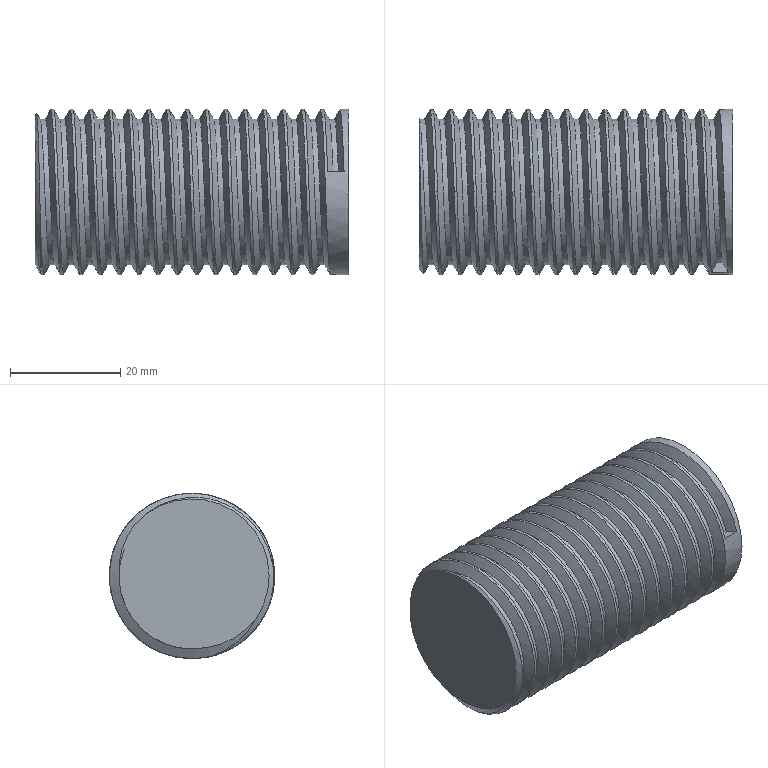Part | STEP file | Tube feed_id662_x_t | 1 solid | 23 faces | box 57 x 30 x 30 mm | volume 35009 mm3 | cylinder 17 | plane 3 | spline 2 | cone 1 | commonest cylinder face diameters 30 x16 26.5 x1